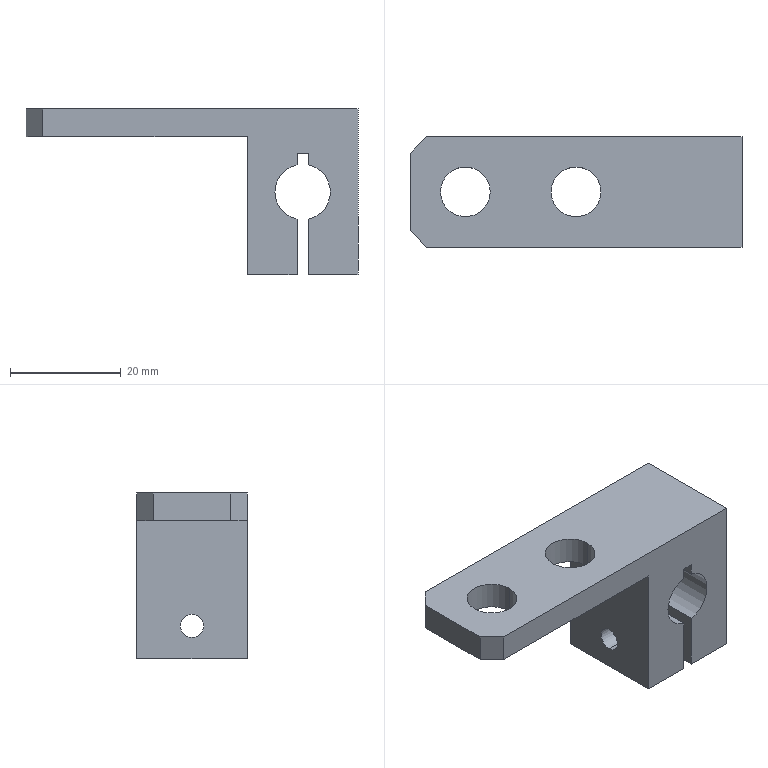Part | SolidWorks | features BaseBody 1 | 1 solid | 30 faces | box 60 x 20 x 30 mm | volume 12631 mm3 | plane 17 | cylinder 13 | commonest cylinder face diameters 10 x5 9 x4 4.2 x2 5.5 x2
STEP:
#1=CARTESIAN_POINT('',(24.6,0.,11.));
#2=VERTEX_POINT('',#1);
#3=CARTESIAN_POINT('',(24.6,0.,1.));
#4=VERTEX_POINT('',#3);
#5=CARTESIAN_POINT('',(24.6,0.,6.));
#6=DIRECTION('',(1.,0.,0.));
#7=DIRECTION('',(0.,0.,-1.));
#8=AXIS2_PLACEMENT_3D('',#5,#6,#7);
#9=CIRCLE('',#8,5.);
#10=EDGE_CURVE('',#2,#4,#9,.T.);
#11=ORIENTED_EDGE('',*,*,#10,.F.);
#12=CARTESIAN_POINT('',(30.,0.,11.));
#13=VERTEX_POINT('',#12);
#14=CARTESIAN_POINT('',(30.,0.,11.));
#15=DIRECTION('',(1.,0.,0.));
#16=VECTOR('',#15,1000.);
#17=LINE('',#14,#16);
#18=EDGE_CURVE('',#2,#13,#17,.T.);
#19=ORIENTED_EDGE('',*,*,#18,.T.);
#20=CARTESIAN_POINT('',(30.,0.,1.));
#21=VERTEX_POINT('',#20);
#22=CARTESIAN_POINT('',(30.,0.,6.));
#23=DIRECTION('',(1.,0.,0.));
#24=DIRECTION('',(0.,0.,-1.));
#25=AXIS2_PLACEMENT_3D('',#22,#23,#24);
#26=CIRCLE('',#25,5.);
#27=EDGE_CURVE('',#13,#21,#26,.T.);
#28=ORIENTED_EDGE('',*,*,#27,.T.);
#29=CARTESIAN_POINT('',(30.,0.,1.));
#30=DIRECTION('',(1.,0.,0.));
#31=VECTOR('',#30,1000.);
#32=LINE('',#29,#31);
#33=EDGE_CURVE('',#4,#21,#32,.T.);
#34=ORIENTED_EDGE('',*,*,#33,.F.);
#35=EDGE_LOOP('',(#11,#19,#28,#34));
#36=FACE_OUTER_BOUND('',#35,.T.);
#37=CARTESIAN_POINT('',(30.,0.,6.));
#38=DIRECTION('',(1.,0.,0.));
#39=DIRECTION('',(0.,0.,-1.));
#40=AXIS2_PLACEMENT_3D('',#37,#38,#39);
#41=CYLINDRICAL_SURFACE('',#40,5.);
#42=ADVANCED_FACE('',(#36),#41,.F.);
#43=CARTESIAN_POINT('',(21.,0.,3.25));
#44=VERTEX_POINT('',#43);
#45=CARTESIAN_POINT('',(21.,0.,8.75));
#46=VERTEX_POINT('',#45);
#47=CARTESIAN_POINT('',(21.,0.,6.));
#48=DIRECTION('',(-1.,0.,0.));
#49=DIRECTION('',(0.,1.,0.));
#50=AXIS2_PLACEMENT_3D('',#47,#48,#49);
#51=CIRCLE('',#50,2.75);
#52=EDGE_CURVE('',#44,#46,#51,.T.);
#53=ORIENTED_EDGE('',*,*,#52,.T.);
#54=CARTESIAN_POINT('',(24.6,0.,8.75));
#55=VERTEX_POINT('',#54);
#56=CARTESIAN_POINT('',(30.,0.,8.75));
#57=DIRECTION('',(1.,0.,0.));
#58=VECTOR('',#57,1000.);
#59=LINE('',#56,#58);
#60=EDGE_CURVE('',#46,#55,#59,.T.);
#61=ORIENTED_EDGE('',*,*,#60,.T.);
#62=CARTESIAN_POINT('',(24.6,0.,3.25));
#63=VERTEX_POINT('',#62);
#64=CARTESIAN_POINT('',(24.6,0.,6.));
#65=DIRECTION('',(1.,0.,0.));
#66=DIRECTION('',(0.,0.,-1.));
#67=AXIS2_PLACEMENT_3D('',#64,#65,#66);
#68=CIRCLE('',#67,2.75);
#69=EDGE_CURVE('',#55,#63,#68,.T.);
#70=ORIENTED_EDGE('',*,*,#69,.T.);
#71=CARTESIAN_POINT('',(30.,0.,3.25));
#72=DIRECTION('',(1.,0.,0.));
#73=VECTOR('',#72,1000.);
#74=LINE('',#71,#73);
#75=EDGE_CURVE('',#44,#63,#74,.T.);
#76=ORIENTED_EDGE('',*,*,#75,.F.);
#77=EDGE_LOOP('',(#53,#61,#70,#76));
#78=FACE_OUTER_BOUND('',#77,.T.);
#79=CARTESIAN_POINT('',(30.,0.,6.));
#80=DIRECTION('',(1.,0.,0.));
#81=DIRECTION('',(0.,0.,-1.));
#82=AXIS2_PLACEMENT_3D('',#79,#80,#81);
#83=CYLINDRICAL_SURFACE('',#82,2.75);
#84=ADVANCED_FACE('',(#78),#83,.F.);
#85=CARTESIAN_POINT('',(10.,0.,8.1));
#86=VERTEX_POINT('',#85);
#87=CARTESIAN_POINT('',(10.,0.,3.9));
#88=VERTEX_POINT('',#87);
#89=CARTESIAN_POINT('',(10.,0.,6.));
#90=DIRECTION('',(1.,0.,0.));
#91=DIRECTION('',(0.,1.,0.));
#92=AXIS2_PLACEMENT_3D('',#89,#90,#91);
#93=CIRCLE('',#92,2.1);
#94=EDGE_CURVE('',#86,#88,#93,.T.);
#95=ORIENTED_EDGE('',*,*,#94,.F.);
#96=CARTESIAN_POINT('',(19.,0.,8.1));
#97=VERTEX_POINT('',#96);
#98=CARTESIAN_POINT('',(19.,0.,8.1));
#99=DIRECTION('',(1.,0.,0.));
#100=VECTOR('',#99,1000.);
#101=LINE('',#98,#100);
#102=EDGE_CURVE('',#86,#97,#101,.T.);
#103=ORIENTED_EDGE('',*,*,#102,.T.);
#104=CARTESIAN_POINT('',(19.,0.,3.9));
#105=VERTEX_POINT('',#104);
#106=CARTESIAN_POINT('',(19.,0.,6.));
#107=DIRECTION('',(1.,0.,0.));
#108=DIRECTION('',(0.,0.,-1.));
#109=AXIS2_PLACEMENT_3D('',#106,#107,#108);
#110=CIRCLE('',#109,2.1);
#111=EDGE_CURVE('',#97,#105,#110,.T.);
#112=ORIENTED_EDGE('',*,*,#111,.T.);
#113=CARTESIAN_POINT('',(19.,0.,3.9));
#114=DIRECTION('',(1.,0.,0.));
#115=VECTOR('',#114,1000.);
#116=LINE('',#113,#115);
#117=EDGE_CURVE('',#88,#105,#116,.T.);
#118=ORIENTED_EDGE('',*,*,#117,.F.);
#119=EDGE_LOOP('',(#95,#103,#112,#118));
#120=FACE_OUTER_BOUND('',#119,.T.);
#121=CARTESIAN_POINT('',(19.,0.,6.));
#122=DIRECTION('',(1.,0.,0.));
#123=DIRECTION('',(0.,0.,-1.));
#124=AXIS2_PLACEMENT_3D('',#121,#122,#123);
#125=CYLINDRICAL_SURFACE('',#124,2.1);
#126=ADVANCED_FACE('',(#120),#125,.F.);
#127=CARTESIAN_POINT('',(-24.5,0.,30.));
#128=VERTEX_POINT('',#127);
#129=CARTESIAN_POINT('',(-15.5,0.,30.));
#130=VERTEX_POINT('',#129);
#131=CARTESIAN_POINT('',(-20.,0.,30.));
#132=DIRECTION('',(0.,0.,1.));
#133=DIRECTION('',(1.,0.,0.));
#134=AXIS2_PLACEMENT_3D('',#131,#132,#133);
#135=CIRCLE('',#134,4.5);
#136=EDGE_CURVE('',#128,#130,#135,.T.);
#137=ORIENTED_EDGE('',*,*,#136,.T.);
#138=CARTESIAN_POINT('',(-15.5,0.,25.));
#139=VERTEX_POINT('',#138);
#140=CARTESIAN_POINT('',(-15.5,0.,25.));
#141=DIRECTION('',(0.,0.,-1.));
#142=VECTOR('',#141,1000.);
#143=LINE('',#140,#142);
#144=EDGE_CURVE('',#130,#139,#143,.T.);
#145=ORIENTED_EDGE('',*,*,#144,.T.);
#146=CARTESIAN_POINT('',(-24.5,0.,25.));
#147=VERTEX_POINT('',#146);
#148=CARTESIAN_POINT('',(-20.,0.,25.));
#149=DIRECTION('',(0.,0.,-1.));
#150=DIRECTION('',(-1.,0.,0.));
#151=AXIS2_PLACEMENT_3D('',#148,#149,#150);
#152=CIRCLE('',#151,4.5);
#153=EDGE_CURVE('',#139,#147,#152,.T.);
#154=ORIENTED_EDGE('',*,*,#153,.T.);
#155=CARTESIAN_POINT('',(-24.5,0.,25.));
#156=DIRECTION('',(0.,0.,-1.));
#157=VECTOR('',#156,1000.);
#158=LINE('',#155,#157);
#159=EDGE_CURVE('',#128,#147,#158,.T.);
#160=ORIENTED_EDGE('',*,*,#159,.F.);
#161=EDGE_LOOP('',(#137,#145,#154,#160));
#162=FACE_OUTER_BOUND('',#161,.T.);
#163=CARTESIAN_POINT('',(-20.,0.,25.));
#164=DIRECTION('',(0.,0.,-1.));
#165=DIRECTION('',(-1.,0.,0.));
#166=AXIS2_PLACEMENT_3D('',#163,#164,#165);
#167=CYLINDRICAL_SURFACE('',#166,4.5);
#168=ADVANCED_FACE('',(#162),#167,.F.);
#169=CARTESIAN_POINT('',(-4.5,0.,30.));
#170=VERTEX_POINT('',#169);
#171=CARTESIAN_POINT('',(4.5,0.,30.));
#172=VERTEX_POINT('',#171);
#173=CARTESIAN_POINT('',(0.,0.,30.));
#174=DIRECTION('',(0.,0.,1.));
#175=DIRECTION('',(1.,0.,0.));
#176=AXIS2_PLACEMENT_3D('',#173,#174,#175);
#177=CIRCLE('',#176,4.5);
#178=EDGE_CURVE('',#170,#172,#177,.T.);
#179=ORIENTED_EDGE('',*,*,#178,.T.);
#180=CARTESIAN_POINT('',(4.5,0.,25.));
#181=VERTEX_POINT('',#180);
#182=CARTESIAN_POINT('',(4.5,0.,25.));
#183=DIRECTION('',(0.,0.,-1.));
#184=VECTOR('',#183,1000.);
#185=LINE('',#182,#184);
#186=EDGE_CURVE('',#172,#181,#185,.T.);
#187=ORIENTED_EDGE('',*,*,#186,.T.);
#188=CARTESIAN_POINT('',(-4.5,0.,25.));
#189=VERTEX_POINT('',#188);
#190=CARTESIAN_POINT('',(0.,0.,25.));
#191=DIRECTION('',(0.,0.,-1.));
#192=DIRECTION('',(-1.,0.,0.));
#193=AXIS2_PLACEMENT_3D('',#190,#191,#192);
#194=CIRCLE('',#193,4.5);
#195=EDGE_CURVE('',#181,#189,#194,.T.);
#196=ORIENTED_EDGE('',*,*,#195,.T.);
#197=CARTESIAN_POINT('',(-4.5,0.,25.));
#198=DIRECTION('',(0.,0.,-1.));
#199=VECTOR('',#198,1000.);
#200=LINE('',#197,#199);
#201=EDGE_CURVE('',#170,#189,#200,.T.);
#202=ORIENTED_EDGE('',*,*,#201,.F.);
#203=EDGE_LOOP('',(#179,#187,#196,#202));
#204=FACE_OUTER_BOUND('',#203,.T.);
#205=CARTESIAN_POINT('',(0.,0.,25.));
#206=DIRECTION('',(0.,0.,-1.));
#207=DIRECTION('',(-1.,0.,0.));
#208=AXIS2_PLACEMENT_3D('',#205,#206,#207);
#209=CYLINDRICAL_SURFACE('',#208,4.5);
#210=ADVANCED_FACE('',(#204),#209,.F.);
#211=CARTESIAN_POINT('',(15.,-10.,15.));
#212=VERTEX_POINT('',#211);
#213=CARTESIAN_POINT('',(19.,-10.,19.899));
#214=VERTEX_POINT('',#213);
#215=CARTESIAN_POINT('',(20.,-10.,15.));
#216=DIRECTION('',(0.,1.,0.));
#217=DIRECTION('',(-1.,0.,0.));
#218=AXIS2_PLACEMENT_3D('',#215,#216,#217);
#219=CIRCLE('',#218,5.);
#220=EDGE_CURVE('',#212,#214,#219,.T.);
#221=ORIENTED_EDGE('',*,*,#220,.F.);
#222=CARTESIAN_POINT('',(15.,10.,15.));
#223=VERTEX_POINT('',#222);
#224=CARTESIAN_POINT('',(15.,-10.,15.));
#225=DIRECTION('',(0.,1.,0.));
#226=VECTOR('',#225,1000.);
#227=LINE('',#224,#226);
#228=EDGE_CURVE('',#212,#223,#227,.T.);
#229=ORIENTED_EDGE('',*,*,#228,.T.);
#230=CARTESIAN_POINT('',(19.,10.,19.899));
#231=VERTEX_POINT('',#230);
#232=CARTESIAN_POINT('',(20.,10.,15.));
#233=DIRECTION('',(0.,1.,0.));
#234=DIRECTION('',(-1.,0.,0.));
#235=AXIS2_PLACEMENT_3D('',#232,#233,#234);
#236=CIRCLE('',#235,5.);
#237=EDGE_CURVE('',#223,#231,#236,.T.);
#238=ORIENTED_EDGE('',*,*,#237,.T.);
#239=CARTESIAN_POINT('',(19.,-10.,19.899));
#240=DIRECTION('',(0.,-1.,0.));
#241=VECTOR('',#240,1000.);
#242=LINE('',#239,#241);
#243=EDGE_CURVE('',#231,#214,#242,.T.);
#244=ORIENTED_EDGE('',*,*,#243,.T.);
#245=EDGE_LOOP('',(#221,#229,#238,#244));
#246=FACE_OUTER_BOUND('',#245,.T.);
#247=CARTESIAN_POINT('',(20.,-10.,15.));
#248=DIRECTION('',(0.,1.,0.));
#249=DIRECTION('',(-1.,0.,0.));
#250=AXIS2_PLACEMENT_3D('',#247,#248,#249);
#251=CYLINDRICAL_SURFACE('',#250,5.);
#252=ADVANCED_FACE('',(#246),#251,.F.);
#253=CARTESIAN_POINT('',(21.,10.,0.));
#254=VERTEX_POINT('',#253);
#255=CARTESIAN_POINT('',(21.,10.,10.101));
#256=VERTEX_POINT('',#255);
#257=CARTESIAN_POINT('',(21.,10.,22.));
#258=DIRECTION('',(0.,0.,1.));
#259=VECTOR('',#258,1000.);
#260=LINE('',#257,#259);
#261=EDGE_CURVE('',#254,#256,#260,.T.);
#262=ORIENTED_EDGE('',*,*,#261,.F.);
#263=CARTESIAN_POINT('',(21.,-10.,0.));
#264=VERTEX_POINT('',#263);
#265=CARTESIAN_POINT('',(21.,10.,0.));
#266=DIRECTION('',(0.,-1.,0.));
#267=VECTOR('',#266,1000.);
#268=LINE('',#265,#267);
#269=EDGE_CURVE('',#254,#264,#268,.T.);
#270=ORIENTED_EDGE('',*,*,#269,.T.);
#271=CARTESIAN_POINT('',(21.,-10.,10.101));
#272=VERTEX_POINT('',#271);
#273=CARTESIAN_POINT('',(21.,-10.,22.));
#274=DIRECTION('',(0.,0.,1.));
#275=VECTOR('',#274,1000.);
#276=LINE('',#273,#275);
#277=EDGE_CURVE('',#264,#272,#276,.T.);
#278=ORIENTED_EDGE('',*,*,#277,.T.);
#279=CARTESIAN_POINT('',(21.,-10.,10.101));
#280=DIRECTION('',(0.,-1.,0.));
#281=VECTOR('',#280,1000.);
#282=LINE('',#279,#281);
#283=EDGE_CURVE('',#256,#272,#282,.T.);
#284=ORIENTED_EDGE('',*,*,#283,.F.);
#285=EDGE_LOOP('',(#262,#270,#278,#284));
#286=FACE_OUTER_BOUND('',#285,.T.);
#287=ORIENTED_EDGE('',*,*,#52,.F.);
#288=CARTESIAN_POINT('',(21.,0.,6.));
#289=DIRECTION('',(-1.,0.,0.));
#290=DIRECTION('',(0.,1.,0.));
#291=AXIS2_PLACEMENT_3D('',#288,#289,#290);
#292=CIRCLE('',#291,2.75);
#293=EDGE_CURVE('',#46,#44,#292,.T.);
#294=ORIENTED_EDGE('',*,*,#293,.F.);
#295=EDGE_LOOP('',(#287,#294));
#296=FACE_BOUND('',#295,.T.);
#297=CARTESIAN_POINT('',(21.,10.,22.));
#298=DIRECTION('',(1.,0.,0.));
#299=DIRECTION('',(0.,1.,0.));
#300=AXIS2_PLACEMENT_3D('',#297,#298,#299);
#301=PLANE('',#300);
#302=ADVANCED_FACE('',(#286,#296),#301,.F.);
#303=CARTESIAN_POINT('',(19.,10.,0.));
#304=VERTEX_POINT('',#303);
#305=CARTESIAN_POINT('',(10.,10.,0.));
#306=VERTEX_POINT('',#305);
#307=CARTESIAN_POINT('',(30.,10.,0.));
#308=DIRECTION('',(-1.,0.,0.));
#309=VECTOR('',#308,1000.);
#310=LINE('',#307,#309);
#311=EDGE_CURVE('',#304,#306,#310,.T.);
#312=ORIENTED_EDGE('',*,*,#311,.F.);
#313=CARTESIAN_POINT('',(19.,-10.,0.));
#314=VERTEX_POINT('',#313);
#315=CARTESIAN_POINT('',(19.,10.,0.));
#316=DIRECTION('',(0.,-1.,0.));
#317=VECTOR('',#316,1000.);
#318=LINE('',#315,#317);
#319=EDGE_CURVE('',#304,#314,#318,.T.);
#320=ORIENTED_EDGE('',*,*,#319,.T.);
#321=CARTESIAN_POINT('',(10.,-10.,0.));
#322=VERTEX_POINT('',#321);
#323=CARTESIAN_POINT('',(30.,-10.,0.));
#324=DIRECTION('',(1.,0.,0.));
#325=VECTOR('',#324,1000.);
#326=LINE('',#323,#325);
#327=EDGE_CURVE('',#322,#314,#326,.T.);
#328=ORIENTED_EDGE('',*,*,#327,.F.);
#329=CARTESIAN_POINT('',(10.,-10.,0.));
#330=DIRECTION('',(0.,1.,0.));
#331=VECTOR('',#330,1000.);
#332=LINE('',#329,#331);
#333=EDGE_CURVE('',#322,#306,#332,.T.);
#334=ORIENTED_EDGE('',*,*,#333,.T.);
#335=EDGE_LOOP('',(#312,#320,#328,#334));
#336=FACE_OUTER_BOUND('',#335,.T.);
#337=CARTESIAN_POINT('',(0.,0.,0.));
#338=DIRECTION('',(0.,0.,1.));
#339=DIRECTION('',(1.,0.,0.));
#340=AXIS2_PLACEMENT_3D('',#337,#338,#339);
#341=PLANE('',#340);
#342=ADVANCED_FACE('',(#336),#341,.F.);
#343=ORIENTED_EDGE('',*,*,#228,.F.);
#344=CARTESIAN_POINT('',(19.,-10.,10.101));
#345=VERTEX_POINT('',#344);
#346=CARTESIAN_POINT('',(20.,-10.,15.));
#347=DIRECTION('',(0.,1.,0.));
#348=DIRECTION('',(-1.,0.,0.));
#349=AXIS2_PLACEMENT_3D('',#346,#347,#348);
#350=CIRCLE('',#349,5.);
#351=EDGE_CURVE('',#345,#212,#350,.T.);
#352=ORIENTED_EDGE('',*,*,#351,.F.);
#353=CARTESIAN_POINT('',(19.,10.,10.101));
#354=VERTEX_POINT('',#353);
#355=CARTESIAN_POINT('',(19.,-10.,10.101));
#356=DIRECTION('',(0.,1.,0.));
#357=VECTOR('',#356,1000.);
#358=LINE('',#355,#357);
#359=EDGE_CURVE('',#345,#354,#358,.T.);
#360=ORIENTED_EDGE('',*,*,#359,.T.);
#361=CARTESIAN_POINT('',(20.,10.,15.));
#362=DIRECTION('',(0.,1.,0.));
#363=DIRECTION('',(-1.,0.,0.));
#364=AXIS2_PLACEMENT_3D('',#361,#362,#363);
#365=CIRCLE('',#364,5.);
#366=EDGE_CURVE('',#354,#223,#365,.T.);
#367=ORIENTED_EDGE('',*,*,#366,.T.);
#368=EDGE_LOOP('',(#343,#352,#360,#367));
#369=FACE_OUTER_BOUND('',#368,.T.);
#370=CARTESIAN_POINT('',(20.,-10.,15.));
#371=DIRECTION('',(0.,1.,0.));
#372=DIRECTION('',(-1.,0.,0.));
#373=AXIS2_PLACEMENT_3D('',#370,#371,#372);
#374=CYLINDRICAL_SURFACE('',#373,5.);
#375=ADVANCED_FACE('',(#369),#374,.F.);
#376=CARTESIAN_POINT('',(-30.,-7.,25.));
#377=VERTEX_POINT('',#376);
#378=CARTESIAN_POINT('',(-30.,7.,25.));
#379=VERTEX_POINT('',#378);
#380=CARTESIAN_POINT('',(-30.,-10.,25.));
#381=DIRECTION('',(0.,1.,0.));
#382=VECTOR('',#381,1000.);
#383=LINE('',#380,#382);
#384=EDGE_CURVE('',#377,#379,#383,.T.);
#385=ORIENTED_EDGE('',*,*,#384,.F.);
#386=CARTESIAN_POINT('',(-30.,-7.,30.));
#387=VERTEX_POINT('',#386);
#388=CARTESIAN_POINT('',(-30.,-7.,30.));
#389=DIRECTION('',(0.,0.,1.));
#390=VECTOR('',#389,1000.);
#391=LINE('',#388,#390);
#392=EDGE_CURVE('',#377,#387,#391,.T.);
#393=ORIENTED_EDGE('',*,*,#392,.T.);
#394=CARTESIAN_POINT('',(-30.,7.,30.));
#395=VERTEX_POINT('',#394);
#396=CARTESIAN_POINT('',(-30.,-10.,30.));
#397=DIRECTION('',(0.,-1.,0.));
#398=VECTOR('',#397,1000.);
#399=LINE('',#396,#398);
#400=EDGE_CURVE('',#395,#387,#399,.T.);
#401=ORIENTED_EDGE('',*,*,#400,.F.);
#402=CARTESIAN_POINT('',(-30.,7.,30.));
#403=DIRECTION('',(0.,0.,-1.));
#404=VECTOR('',#403,1000.);
#405=LINE('',#402,#404);
#406=EDGE_CURVE('',#395,#379,#405,.T.);
#407=ORIENTED_EDGE('',*,*,#406,.T.);
#408=EDGE_LOOP('',(#385,#393,#401,#407));
#409=FACE_OUTER_BOUND('',#408,.T.);
#410=CARTESIAN_POINT('',(-30.,-10.,30.));
#411=DIRECTION('',(1.,0.,0.));
#412=DIRECTION('',(0.,0.,-1.));
#413=AXIS2_PLACEMENT_3D('',#410,#411,#412);
#414=PLANE('',#413);
#415=ADVANCED_FACE('',(#409),#414,.F.);
#416=ORIENTED_EDGE('',*,*,#327,.T.);
#417=CARTESIAN_POINT('',(19.,-10.,22.));
#418=DIRECTION('',(0.,0.,-1.));
#419=VECTOR('',#418,1000.);
#420=LINE('',#417,#419);
#421=EDGE_CURVE('',#345,#314,#420,.T.);
#422=ORIENTED_EDGE('',*,*,#421,.F.);
#423=ORIENTED_EDGE('',*,*,#351,.T.);
#424=ORIENTED_EDGE('',*,*,#220,.T.);
#425=CARTESIAN_POINT('',(19.,-10.,22.));
#426=VERTEX_POINT('',#425);
#427=CARTESIAN_POINT('',(19.,-10.,22.));
#428=DIRECTION('',(0.,0.,-1.));
#429=VECTOR('',#428,1000.);
#430=LINE('',#427,#429);
#431=EDGE_CURVE('',#426,#214,#430,.T.);
#432=ORIENTED_EDGE('',*,*,#431,.F.);
#433=CARTESIAN_POINT('',(21.,-10.,22.));
#434=VERTEX_POINT('',#433);
#435=CARTESIAN_POINT('',(19.,-10.,22.));
#436=DIRECTION('',(-1.,0.,0.));
#437=VECTOR('',#436,1000.);
#438=LINE('',#435,#437);
#439=EDGE_CURVE('',#434,#426,#438,.T.);
#440=ORIENTED_EDGE('',*,*,#439,.F.);
#441=CARTESIAN_POINT('',(21.,-10.,19.899));
#442=VERTEX_POINT('',#441);
#443=CARTESIAN_POINT('',(21.,-10.,22.));
#444=DIRECTION('',(0.,0.,1.));
#445=VECTOR('',#444,1000.);
#446=LINE('',#443,#445);
#447=EDGE_CURVE('',#442,#434,#446,.T.);
#448=ORIENTED_EDGE('',*,*,#447,.F.);
#449=CARTESIAN_POINT('',(20.,-10.,15.));
#450=DIRECTION('',(0.,1.,0.));
#451=DIRECTION('',(-1.,0.,0.));
#452=AXIS2_PLACEMENT_3D('',#449,#450,#451);
#453=CIRCLE('',#452,5.);
#454=EDGE_CURVE('',#442,#272,#453,.T.);
#455=ORIENTED_EDGE('',*,*,#454,.T.);
#456=ORIENTED_EDGE('',*,*,#277,.F.);
#457=CARTESIAN_POINT('',(30.,-10.,0.));
#458=VERTEX_POINT('',#457);
#459=CARTESIAN_POINT('',(30.,-10.,0.));
#460=DIRECTION('',(1.,0.,0.));
#461=VECTOR('',#460,1000.);
#462=LINE('',#459,#461);
#463=EDGE_CURVE('',#264,#458,#462,.T.);
#464=ORIENTED_EDGE('',*,*,#463,.T.);
#465=CARTESIAN_POINT('',(30.,-10.,30.));
#466=VERTEX_POINT('',#465);
#467=CARTESIAN_POINT('',(30.,-10.,30.));
#468=DIRECTION('',(0.,0.,-1.));
#469=VECTOR('',#468,1000.);
#470=LINE('',#467,#469);
#471=EDGE_CURVE('',#466,#458,#470,.T.);
#472=ORIENTED_EDGE('',*,*,#471,.F.);
#473=CARTESIAN_POINT('',(-27.,-10.,30.));
#474=VERTEX_POINT('',#473);
#475=CARTESIAN_POINT('',(30.,-10.,30.));
#476=DIRECTION('',(1.,0.,0.));
#477=VECTOR('',#476,1000.);
#478=LINE('',#475,#477);
#479=EDGE_CURVE('',#474,#466,#478,.T.);
#480=ORIENTED_EDGE('',*,*,#479,.F.);
#481=CARTESIAN_POINT('',(-27.,-10.,25.));
#482=VERTEX_POINT('',#481);
#483=CARTESIAN_POINT('',(-27.,-10.,30.));
#484=DIRECTION('',(0.,0.,-1.));
#485=VECTOR('',#484,1000.);
#486=LINE('',#483,#485);
#487=EDGE_CURVE('',#474,#482,#486,.T.);
#488=ORIENTED_EDGE('',*,*,#487,.T.);
#489=CARTESIAN_POINT('',(10.,-10.,25.));
#490=VERTEX_POINT('',#489);
#491=CARTESIAN_POINT('',(-30.,-10.,25.));
#492=DIRECTION('',(1.,0.,0.));
#493=VECTOR('',#492,1000.);
#494=LINE('',#491,#493);
#495=EDGE_CURVE('',#482,#490,#494,.T.);
#496=ORIENTED_EDGE('',*,*,#495,.T.);
#497=CARTESIAN_POINT('',(10.,-10.,25.));
#498=DIRECTION('',(0.,0.,-1.));
#499=VECTOR('',#498,1000.);
#500=LINE('',#497,#499);
#501=EDGE_CURVE('',#490,#322,#500,.T.);
#502=ORIENTED_EDGE('',*,*,#501,.T.);
#503=EDGE_LOOP('',(#416,#422,#423,#424,#432,#440,#448,#455,#456,#464,#472,#480,#488,#496,#502));
#504=FACE_OUTER_BOUND('',#503,.T.);
#505=CARTESIAN_POINT('',(30.,-10.,30.));
#506=DIRECTION('',(0.,1.,0.));
#507=DIRECTION('',(-1.,0.,0.));
#508=AXIS2_PLACEMENT_3D('',#505,#506,#507);
#509=PLANE('',#508);
#510=ADVANCED_FACE('',(#504),#509,.F.);
#511=CARTESIAN_POINT('',(30.,0.,6.));
#512=DIRECTION('',(1.,0.,0.));
#513=DIRECTION('',(0.,0.,-1.));
#514=AXIS2_PLACEMENT_3D('',#511,#512,#513);
#515=CIRCLE('',#514,5.);
#516=EDGE_CURVE('',#21,#13,#515,.T.);
#517=ORIENTED_EDGE('',*,*,#516,.F.);
#518=ORIENTED_EDGE('',*,*,#27,.F.);
#519=EDGE_LOOP('',(#517,#518));
#520=FACE_BOUND('',#519,.T.);
#521=CARTESIAN_POINT('',(30.,10.,0.));
#522=VERTEX_POINT('',#521);
#523=CARTESIAN_POINT('',(30.,-10.,0.));
#524=DIRECTION('',(0.,1.,0.));
#525=VECTOR('',#524,1000.);
#526=LINE('',#523,#525);
#527=EDGE_CURVE('',#458,#522,#526,.T.);
#528=ORIENTED_EDGE('',*,*,#527,.T.);
#529=CARTESIAN_POINT('',(30.,10.,30.));
#530=VERTEX_POINT('',#529);
#531=CARTESIAN_POINT('',(30.,10.,30.));
#532=DIRECTION('',(0.,0.,-1.));
#533=VECTOR('',#532,1000.);
#534=LINE('',#531,#533);
#535=EDGE_CURVE('',#530,#522,#534,.T.);
#536=ORIENTED_EDGE('',*,*,#535,.F.);
#537=CARTESIAN_POINT('',(30.,-10.,30.));
#538=DIRECTION('',(0.,1.,0.));
#539=VECTOR('',#538,1000.);
#540=LINE('',#537,#539);
#541=EDGE_CURVE('',#466,#530,#540,.T.);
#542=ORIENTED_EDGE('',*,*,#541,.F.);
#543=ORIENTED_EDGE('',*,*,#471,.T.);
#544=EDGE_LOOP('',(#528,#536,#542,#543));
#545=FACE_OUTER_BOUND('',#544,.T.);
#546=CARTESIAN_POINT('',(30.,-10.,30.));
#547=DIRECTION('',(-1.,0.,0.));
#548=DIRECTION('',(0.,0.,1.));
#549=AXIS2_PLACEMENT_3D('',#546,#547,#548);
#550=PLANE('',#549);
#551=ADVANCED_FACE('',(#520,#545),#550,.F.);
#552=ORIENTED_EDGE('',*,*,#366,.F.);
#553=CARTESIAN_POINT('',(19.,10.,22.));
#554=DIRECTION('',(0.,0.,-1.));
#555=VECTOR('',#554,1000.);
#556=LINE('',#553,#555);
#557=EDGE_CURVE('',#354,#304,#556,.T.);
#558=ORIENTED_EDGE('',*,*,#557,.T.);
#559=ORIENTED_EDGE('',*,*,#311,.T.);
#560=CARTESIAN_POINT('',(10.,10.,25.));
#561=VERTEX_POINT('',#560);
#562=CARTESIAN_POINT('',(10.,10.,25.));
#563=DIRECTION('',(0.,0.,-1.));
#564=VECTOR('',#563,1000.);
#565=LINE('',#562,#564);
#566=EDGE_CURVE('',#561,#306,#565,.T.);
#567=ORIENTED_EDGE('',*,*,#566,.F.);
#568=CARTESIAN_POINT('',(-27.,10.,25.));
#569=VERTEX_POINT('',#568);
#570=CARTESIAN_POINT('',(-30.,10.,25.));
#571=DIRECTION('',(1.,0.,0.));
#572=VECTOR('',#571,1000.);
#573=LINE('',#570,#572);
#574=EDGE_CURVE('',#569,#561,#573,.T.);
#575=ORIENTED_EDGE('',*,*,#574,.F.);
#576=CARTESIAN_POINT('',(-27.,10.,30.));
#577=VERTEX_POINT('',#576);
#578=CARTESIAN_POINT('',(-27.,10.,30.));
#579=DIRECTION('',(0.,0.,1.));
#580=VECTOR('',#579,1000.);
#581=LINE('',#578,#580);
#582=EDGE_CURVE('',#569,#577,#581,.T.);
#583=ORIENTED_EDGE('',*,*,#582,.T.);
#584=CARTESIAN_POINT('',(30.,10.,30.));
#585=DIRECTION('',(-1.,0.,0.));
#586=VECTOR('',#585,1000.);
#587=LINE('',#584,#586);
#588=EDGE_CURVE('',#530,#577,#587,.T.);
#589=ORIENTED_EDGE('',*,*,#588,.F.);
#590=ORIENTED_EDGE('',*,*,#535,.T.);
#591=CARTESIAN_POINT('',(30.,10.,0.));
#592=DIRECTION('',(-1.,0.,0.));
#593=VECTOR('',#592,1000.);
#594=LINE('',#591,#593);
#595=EDGE_CURVE('',#522,#254,#594,.T.);
#596=ORIENTED_EDGE('',*,*,#595,.T.);
#597=ORIENTED_EDGE('',*,*,#261,.T.);
#598=CARTESIAN_POINT('',(21.,10.,19.899));
#599=VERTEX_POINT('',#598);
#600=CARTESIAN_POINT('',(20.,10.,15.));
#601=DIRECTION('',(0.,1.,0.));
#602=DIRECTION('',(-1.,0.,0.));
#603=AXIS2_PLACEMENT_3D('',#600,#601,#602);
#604=CIRCLE('',#603,5.);
#605=EDGE_CURVE('',#599,#256,#604,.T.);
#606=ORIENTED_EDGE('',*,*,#605,.F.);
#607=CARTESIAN_POINT('',(21.,10.,22.));
#608=VERTEX_POINT('',#607);
#609=CARTESIAN_POINT('',(21.,10.,22.));
#610=DIRECTION('',(0.,0.,1.));
#611=VECTOR('',#610,1000.);
#612=LINE('',#609,#611);
#613=EDGE_CURVE('',#599,#608,#612,.T.);
#614=ORIENTED_EDGE('',*,*,#613,.T.);
#615=CARTESIAN_POINT('',(19.,10.,22.));
#616=VERTEX_POINT('',#615);
#617=CARTESIAN_POINT('',(19.,10.,22.));
#618=DIRECTION('',(-1.,0.,0.));
#619=VECTOR('',#618,1000.);
#620=LINE('',#617,#619);
#621=EDGE_CURVE('',#608,#616,#620,.T.);
#622=ORIENTED_EDGE('',*,*,#621,.T.);
#623=CARTESIAN_POINT('',(19.,10.,22.));
#624=DIRECTION('',(0.,0.,-1.));
#625=VECTOR('',#624,1000.);
#626=LINE('',#623,#625);
#627=EDGE_CURVE('',#616,#231,#626,.T.);
#628=ORIENTED_EDGE('',*,*,#627,.T.);
#629=ORIENTED_EDGE('',*,*,#237,.F.);
#630=EDGE_LOOP('',(#552,#558,#559,#567,#575,#583,#589,#590,#596,#597,#606,#614,#622,#628,#629));
#631=FACE_OUTER_BOUND('',#630,.T.);
#632=CARTESIAN_POINT('',(30.,10.,30.));
#633=DIRECTION('',(0.,-1.,0.));
#634=DIRECTION('',(1.,0.,0.));
#635=AXIS2_PLACEMENT_3D('',#632,#633,#634);
#636=PLANE('',#635);
#637=ADVANCED_FACE('',(#631),#636,.F.);
#638=ORIENTED_EDGE('',*,*,#136,.F.);
#639=CARTESIAN_POINT('',(-20.,0.,30.));
#640=DIRECTION('',(0.,0.,1.));
#641=DIRECTION('',(1.,0.,0.));
#642=AXIS2_PLACEMENT_3D('',#639,#640,#641);
#643=CIRCLE('',#642,4.5);
#644=EDGE_CURVE('',#130,#128,#643,.T.);
#645=ORIENTED_EDGE('',*,*,#644,.F.);
#646=EDGE_LOOP('',(#638,#645));
#647=FACE_BOUND('',#646,.T.);
#648=ORIENTED_EDGE('',*,*,#178,.F.);
#649=CARTESIAN_POINT('',(0.,0.,30.));
#650=DIRECTION('',(0.,0.,1.));
#651=DIRECTION('',(1.,0.,0.));
#652=AXIS2_PLACEMENT_3D('',#649,#650,#651);
#653=CIRCLE('',#652,4.5);
#654=EDGE_CURVE('',#172,#170,#653,.T.);
#655=ORIENTED_EDGE('',*,*,#654,.F.);
#656=EDGE_LOOP('',(#648,#655));
#657=FACE_BOUND('',#656,.T.);
#658=ORIENTED_EDGE('',*,*,#400,.T.);
#659=CARTESIAN_POINT('',(-18.5,-18.5,30.));
#660=DIRECTION('',(0.7071,-0.7071,0.));
#661=VECTOR('',#660,1000.);
#662=LINE('',#659,#661);
#663=EDGE_CURVE('',#387,#474,#662,.T.);
#664=ORIENTED_EDGE('',*,*,#663,.T.);
#665=ORIENTED_EDGE('',*,*,#479,.T.);
#666=ORIENTED_EDGE('',*,*,#541,.T.);
#667=ORIENTED_EDGE('',*,*,#588,.T.);
#668=CARTESIAN_POINT('',(-18.5,18.5,30.));
#669=DIRECTION('',(-0.7071,-0.7071,0.));
#670=VECTOR('',#669,1000.);
#671=LINE('',#668,#670);
#672=EDGE_CURVE('',#577,#395,#671,.T.);
#673=ORIENTED_EDGE('',*,*,#672,.T.);
#674=EDGE_LOOP('',(#658,#664,#665,#666,#667,#673));
#675=FACE_OUTER_BOUND('',#674,.T.);
#676=CARTESIAN_POINT('',(0.,0.,30.));
#677=DIRECTION('',(0.,0.,1.));
#678=DIRECTION('',(1.,0.,0.));
#679=AXIS2_PLACEMENT_3D('',#676,#677,#678);
#680=PLANE('',#679);
#681=ADVANCED_FACE('',(#647,#657,#675),#680,.T.);
#682=ORIENTED_EDGE('',*,*,#463,.F.);
#683=ORIENTED_EDGE('',*,*,#269,.F.);
#684=ORIENTED_EDGE('',*,*,#595,.F.);
#685=ORIENTED_EDGE('',*,*,#527,.F.);
#686=EDGE_LOOP('',(#682,#683,#684,#685));
#687=FACE_OUTER_BOUND('',#686,.T.);
#688=CARTESIAN_POINT('',(0.,0.,0.));
#689=DIRECTION('',(0.,0.,1.));
#690=DIRECTION('',(1.,0.,0.));
#691=AXIS2_PLACEMENT_3D('',#688,#689,#690);
#692=PLANE('',#691);
#693=ADVANCED_FACE('',(#687),#692,.F.);
#694=CARTESIAN_POINT('',(10.,0.,6.));
#695=DIRECTION('',(1.,0.,0.));
#696=DIRECTION('',(0.,1.,0.));
#697=AXIS2_PLACEMENT_3D('',#694,#695,#696);
#698=CIRCLE('',#697,2.1);
#699=EDGE_CURVE('',#88,#86,#698,.T.);
#700=ORIENTED_EDGE('',*,*,#699,.T.);
#701=ORIENTED_EDGE('',*,*,#94,.T.);
#702=EDGE_LOOP('',(#700,#701));
#703=FACE_BOUND('',#702,.T.);
#704=ORIENTED_EDGE('',*,*,#566,.T.);
#705=ORIENTED_EDGE('',*,*,#333,.F.);
#706=ORIENTED_EDGE('',*,*,#501,.F.);
#707=CARTESIAN_POINT('',(10.,-10.,25.));
#708=DIRECTION('',(0.,1.,0.));
#709=VECTOR('',#708,1000.);
#710=LINE('',#707,#709);
#711=EDGE_CURVE('',#490,#561,#710,.T.);
#712=ORIENTED_EDGE('',*,*,#711,.T.);
#713=EDGE_LOOP('',(#704,#705,#706,#712));
#714=FACE_OUTER_BOUND('',#713,.T.);
#715=CARTESIAN_POINT('',(10.,-10.,25.));
#716=DIRECTION('',(1.,0.,0.));
#717=DIRECTION('',(0.,1.,0.));
#718=AXIS2_PLACEMENT_3D('',#715,#716,#717);
#719=PLANE('',#718);
#720=ADVANCED_FACE('',(#703,#714),#719,.F.);
#721=CARTESIAN_POINT('',(-20.,0.,25.));
#722=DIRECTION('',(0.,0.,-1.));
#723=DIRECTION('',(-1.,0.,0.));
#724=AXIS2_PLACEMENT_3D('',#721,#722,#723);
#725=CIRCLE('',#724,4.5);
#726=EDGE_CURVE('',#147,#139,#725,.T.);
#727=ORIENTED_EDGE('',*,*,#726,.F.);
#728=ORIENTED_EDGE('',*,*,#153,.F.);
#729=EDGE_LOOP('',(#727,#728));
#730=FACE_BOUND('',#729,.T.);
#731=CARTESIAN_POINT('',(0.,0.,25.));
#732=DIRECTION('',(0.,0.,-1.));
#733=DIRECTION('',(-1.,0.,0.));
#734=AXIS2_PLACEMENT_3D('',#731,#732,#733);
#735=CIRCLE('',#734,4.5);
#736=EDGE_CURVE('',#189,#181,#735,.T.);
#737=ORIENTED_EDGE('',*,*,#736,.F.);
#738=ORIENTED_EDGE('',*,*,#195,.F.);
#739=EDGE_LOOP('',(#737,#738));
#740=FACE_BOUND('',#739,.T.);
#741=ORIENTED_EDGE('',*,*,#495,.F.);
#742=CARTESIAN_POINT('',(-27.,-10.,25.));
#743=DIRECTION('',(-0.7071,0.7071,0.));
#744=VECTOR('',#743,1000.);
#745=LINE('',#742,#744);
#746=EDGE_CURVE('',#482,#377,#745,.T.);
#747=ORIENTED_EDGE('',*,*,#746,.T.);
#748=ORIENTED_EDGE('',*,*,#384,.T.);
#749=CARTESIAN_POINT('',(-30.,7.,25.));
#750=DIRECTION('',(0.7071,0.7071,0.));
#751=VECTOR('',#750,1000.);
#752=LINE('',#749,#751);
#753=EDGE_CURVE('',#379,#569,#752,.T.);
#754=ORIENTED_EDGE('',*,*,#753,.T.);
#755=ORIENTED_EDGE('',*,*,#574,.T.);
#756=ORIENTED_EDGE('',*,*,#711,.F.);
#757=EDGE_LOOP('',(#741,#747,#748,#754,#755,#756));
#758=FACE_OUTER_BOUND('',#757,.T.);
#759=CARTESIAN_POINT('',(-30.,-10.,25.));
#760=DIRECTION('',(0.,0.,1.));
#761=DIRECTION('',(1.,0.,0.));
#762=AXIS2_PLACEMENT_3D('',#759,#760,#761);
#763=PLANE('',#762);
#764=ADVANCED_FACE('',(#730,#740,#758),#763,.F.);
#765=ORIENTED_EDGE('',*,*,#605,.T.);
#766=ORIENTED_EDGE('',*,*,#283,.T.);
#767=ORIENTED_EDGE('',*,*,#454,.F.);
#768=CARTESIAN_POINT('',(21.,-10.,19.899));
#769=DIRECTION('',(0.,1.,0.));
#770=VECTOR('',#769,1000.);
#771=LINE('',#768,#770);
#772=EDGE_CURVE('',#442,#599,#771,.T.);
#773=ORIENTED_EDGE('',*,*,#772,.T.);
#774=EDGE_LOOP('',(#765,#766,#767,#773));
#775=FACE_OUTER_BOUND('',#774,.T.);
#776=CARTESIAN_POINT('',(20.,-10.,15.));
#777=DIRECTION('',(0.,1.,0.));
#778=DIRECTION('',(-1.,0.,0.));
#779=AXIS2_PLACEMENT_3D('',#776,#777,#778);
#780=CYLINDRICAL_SURFACE('',#779,5.);
#781=ADVANCED_FACE('',(#775),#780,.F.);
#782=ORIENTED_EDGE('',*,*,#663,.F.);
#783=ORIENTED_EDGE('',*,*,#392,.F.);
#784=ORIENTED_EDGE('',*,*,#746,.F.);
#785=ORIENTED_EDGE('',*,*,#487,.F.);
#786=EDGE_LOOP('',(#782,#783,#784,#785));
#787=FACE_OUTER_BOUND('',#786,.T.);
#788=CARTESIAN_POINT('',(-27.,-10.,30.));
#789=DIRECTION('',(0.7071,0.7071,0.));
#790=DIRECTION('',(0.,0.,-1.));
#791=AXIS2_PLACEMENT_3D('',#788,#789,#790);
#792=PLANE('',#791);
#793=ADVANCED_FACE('',(#787),#792,.F.);
#794=ORIENTED_EDGE('',*,*,#672,.F.);
#795=ORIENTED_EDGE('',*,*,#582,.F.);
#796=ORIENTED_EDGE('',*,*,#753,.F.);
#797=ORIENTED_EDGE('',*,*,#406,.F.);
#798=EDGE_LOOP('',(#794,#795,#796,#797));
#799=FACE_OUTER_BOUND('',#798,.T.);
#800=CARTESIAN_POINT('',(-30.,7.,30.));
#801=DIRECTION('',(0.7071,-0.7071,0.));
#802=DIRECTION('',(0.,0.,-1.));
#803=AXIS2_PLACEMENT_3D('',#800,#801,#802);
#804=PLANE('',#803);
#805=ADVANCED_FACE('',(#799),#804,.F.);
#806=ORIENTED_EDGE('',*,*,#186,.F.);
#807=ORIENTED_EDGE('',*,*,#654,.T.);
#808=ORIENTED_EDGE('',*,*,#201,.T.);
#809=ORIENTED_EDGE('',*,*,#736,.T.);
#810=EDGE_LOOP('',(#806,#807,#808,#809));
#811=FACE_OUTER_BOUND('',#810,.T.);
#812=CARTESIAN_POINT('',(0.,0.,25.));
#813=DIRECTION('',(0.,0.,-1.));
#814=DIRECTION('',(-1.,0.,0.));
#815=AXIS2_PLACEMENT_3D('',#812,#813,#814);
#816=CYLINDRICAL_SURFACE('',#815,4.5);
#817=ADVANCED_FACE('',(#811),#816,.F.);
#818=ORIENTED_EDGE('',*,*,#144,.F.);
#819=ORIENTED_EDGE('',*,*,#644,.T.);
#820=ORIENTED_EDGE('',*,*,#159,.T.);
#821=ORIENTED_EDGE('',*,*,#726,.T.);
#822=EDGE_LOOP('',(#818,#819,#820,#821));
#823=FACE_OUTER_BOUND('',#822,.T.);
#824=CARTESIAN_POINT('',(-20.,0.,25.));
#825=DIRECTION('',(0.,0.,-1.));
#826=DIRECTION('',(-1.,0.,0.));
#827=AXIS2_PLACEMENT_3D('',#824,#825,#826);
#828=CYLINDRICAL_SURFACE('',#827,4.5);
#829=ADVANCED_FACE('',(#823),#828,.F.);
#830=ORIENTED_EDGE('',*,*,#627,.F.);
#831=CARTESIAN_POINT('',(19.,10.,22.));
#832=DIRECTION('',(0.,-1.,0.));
#833=VECTOR('',#832,1000.);
#834=LINE('',#831,#833);
#835=EDGE_CURVE('',#616,#426,#834,.T.);
#836=ORIENTED_EDGE('',*,*,#835,.T.);
#837=ORIENTED_EDGE('',*,*,#431,.T.);
#838=ORIENTED_EDGE('',*,*,#243,.F.);
#839=EDGE_LOOP('',(#830,#836,#837,#838));
#840=FACE_OUTER_BOUND('',#839,.T.);
#841=CARTESIAN_POINT('',(19.,10.,22.));
#842=DIRECTION('',(-1.,0.,0.));
#843=DIRECTION('',(0.,0.,1.));
#844=AXIS2_PLACEMENT_3D('',#841,#842,#843);
#845=PLANE('',#844);
#846=ADVANCED_FACE('',(#840),#845,.F.);
#847=ORIENTED_EDGE('',*,*,#447,.T.);
#848=CARTESIAN_POINT('',(21.,10.,22.));
#849=DIRECTION('',(0.,-1.,0.));
#850=VECTOR('',#849,1000.);
#851=LINE('',#848,#850);
#852=EDGE_CURVE('',#608,#434,#851,.T.);
#853=ORIENTED_EDGE('',*,*,#852,.F.);
#854=ORIENTED_EDGE('',*,*,#613,.F.);
#855=ORIENTED_EDGE('',*,*,#772,.F.);
#856=EDGE_LOOP('',(#847,#853,#854,#855));
#857=FACE_OUTER_BOUND('',#856,.T.);
#858=CARTESIAN_POINT('',(21.,10.,22.));
#859=DIRECTION('',(1.,0.,0.));
#860=DIRECTION('',(0.,1.,0.));
#861=AXIS2_PLACEMENT_3D('',#858,#859,#860);
#862=PLANE('',#861);
#863=ADVANCED_FACE('',(#857),#862,.F.);
#864=ORIENTED_EDGE('',*,*,#439,.T.);
#865=ORIENTED_EDGE('',*,*,#835,.F.);
#866=ORIENTED_EDGE('',*,*,#621,.F.);
#867=ORIENTED_EDGE('',*,*,#852,.T.);
#868=EDGE_LOOP('',(#864,#865,#866,#867));
#869=FACE_OUTER_BOUND('',#868,.T.);
#870=CARTESIAN_POINT('',(19.,10.,22.));
#871=DIRECTION('',(0.,0.,1.));
#872=DIRECTION('',(1.,0.,0.));
#873=AXIS2_PLACEMENT_3D('',#870,#871,#872);
#874=PLANE('',#873);
#875=ADVANCED_FACE('',(#869),#874,.F.);
#876=CARTESIAN_POINT('',(19.,0.,6.));
#877=DIRECTION('',(1.,0.,0.));
#878=DIRECTION('',(0.,0.,-1.));
#879=AXIS2_PLACEMENT_3D('',#876,#877,#878);
#880=CIRCLE('',#879,2.1);
#881=EDGE_CURVE('',#105,#97,#880,.T.);
#882=ORIENTED_EDGE('',*,*,#881,.F.);
#883=ORIENTED_EDGE('',*,*,#111,.F.);
#884=EDGE_LOOP('',(#882,#883));
#885=FACE_BOUND('',#884,.T.);
#886=ORIENTED_EDGE('',*,*,#421,.T.);
#887=ORIENTED_EDGE('',*,*,#319,.F.);
#888=ORIENTED_EDGE('',*,*,#557,.F.);
#889=ORIENTED_EDGE('',*,*,#359,.F.);
#890=EDGE_LOOP('',(#886,#887,#888,#889));
#891=FACE_OUTER_BOUND('',#890,.T.);
#892=CARTESIAN_POINT('',(19.,10.,22.));
#893=DIRECTION('',(-1.,0.,0.));
#894=DIRECTION('',(0.,0.,1.));
#895=AXIS2_PLACEMENT_3D('',#892,#893,#894);
#896=PLANE('',#895);
#897=ADVANCED_FACE('',(#885,#891),#896,.F.);
#898=ORIENTED_EDGE('',*,*,#102,.F.);
#899=ORIENTED_EDGE('',*,*,#699,.F.);
#900=ORIENTED_EDGE('',*,*,#117,.T.);
#901=ORIENTED_EDGE('',*,*,#881,.T.);
#902=EDGE_LOOP('',(#898,#899,#900,#901));
#903=FACE_OUTER_BOUND('',#902,.T.);
#904=CARTESIAN_POINT('',(19.,0.,6.));
#905=DIRECTION('',(1.,0.,0.));
#906=DIRECTION('',(0.,0.,-1.));
#907=AXIS2_PLACEMENT_3D('',#904,#905,#906);
#908=CYLINDRICAL_SURFACE('',#907,2.1);
#909=ADVANCED_FACE('',(#903),#908,.F.);
#910=ORIENTED_EDGE('',*,*,#60,.F.);
#911=ORIENTED_EDGE('',*,*,#293,.T.);
#912=ORIENTED_EDGE('',*,*,#75,.T.);
#913=CARTESIAN_POINT('',(24.6,0.,6.));
#914=DIRECTION('',(1.,0.,0.));
#915=DIRECTION('',(0.,0.,-1.));
#916=AXIS2_PLACEMENT_3D('',#913,#914,#915);
#917=CIRCLE('',#916,2.75);
#918=EDGE_CURVE('',#63,#55,#917,.T.);
#919=ORIENTED_EDGE('',*,*,#918,.T.);
#920=EDGE_LOOP('',(#910,#911,#912,#919));
#921=FACE_OUTER_BOUND('',#920,.T.);
#922=CARTESIAN_POINT('',(30.,0.,6.));
#923=DIRECTION('',(1.,0.,0.));
#924=DIRECTION('',(0.,0.,-1.));
#925=AXIS2_PLACEMENT_3D('',#922,#923,#924);
#926=CYLINDRICAL_SURFACE('',#925,2.75);
#927=ADVANCED_FACE('',(#921),#926,.F.);
#928=ORIENTED_EDGE('',*,*,#918,.F.);
#929=ORIENTED_EDGE('',*,*,#69,.F.);
#930=EDGE_LOOP('',(#928,#929));
#931=FACE_BOUND('',#930,.T.);
#932=CARTESIAN_POINT('',(24.6,0.,6.));
#933=DIRECTION('',(1.,0.,0.));
#934=DIRECTION('',(0.,0.,-1.));
#935=AXIS2_PLACEMENT_3D('',#932,#933,#934);
#936=CIRCLE('',#935,5.);
#937=EDGE_CURVE('',#4,#2,#936,.T.);
#938=ORIENTED_EDGE('',*,*,#937,.T.);
#939=ORIENTED_EDGE('',*,*,#10,.T.);
#940=EDGE_LOOP('',(#938,#939));
#941=FACE_OUTER_BOUND('',#940,.T.);
#942=CARTESIAN_POINT('',(24.6,2.75,6.));
#943=DIRECTION('',(-1.,0.,0.));
#944=DIRECTION('',(0.,0.,1.));
#945=AXIS2_PLACEMENT_3D('',#942,#943,#944);
#946=PLANE('',#945);
#947=ADVANCED_FACE('',(#931,#941),#946,.F.);
#948=ORIENTED_EDGE('',*,*,#18,.F.);
#949=ORIENTED_EDGE('',*,*,#937,.F.);
#950=ORIENTED_EDGE('',*,*,#33,.T.);
#951=ORIENTED_EDGE('',*,*,#516,.T.);
#952=EDGE_LOOP('',(#948,#949,#950,#951));
#953=FACE_OUTER_BOUND('',#952,.T.);
#954=CARTESIAN_POINT('',(30.,0.,6.));
#955=DIRECTION('',(1.,0.,0.));
#956=DIRECTION('',(0.,0.,-1.));
#957=AXIS2_PLACEMENT_3D('',#954,#955,#956);
#958=CYLINDRICAL_SURFACE('',#957,5.);
#959=ADVANCED_FACE('',(#953),#958,.F.);
#960=CLOSED_SHELL('',(#42,#84,#126,#168,#210,#252,#302,#342,#375,#415,#510,#551,#637,#681,#693,#720,#764,#781,#793,#805,#817,#829,#846,#863,#875,#897,#909,#927,#947,#959));
#961=MANIFOLD_SOLID_BREP('',#960);
#962=CARTESIAN_POINT('',(0.,0.,0.));
#963=DIRECTION('',(0.,0.,1.));
#964=DIRECTION('',(1.,0.,0.));
#965=AXIS2_PLACEMENT_3D('',#962,#963,#964);
#966=(LENGTH_UNIT()NAMED_UNIT(*)SI_UNIT(.MILLI.,.METRE.));
#967=UNCERTAINTY_MEASURE_WITH_UNIT(LENGTH_MEASURE(0.00001),#966,'','');
#968=(NAMED_UNIT(*)PLANE_ANGLE_UNIT()SI_UNIT($,.RADIAN.));
#969=(NAMED_UNIT(*)SI_UNIT($,.STERADIAN.)SOLID_ANGLE_UNIT());
#970=(GEOMETRIC_REPRESENTATION_CONTEXT(3)GLOBAL_UNCERTAINTY_ASSIGNED_CONTEXT((#967))GLOBAL_UNIT_ASSIGNED_CONTEXT((#966,#968,#969))REPRESENTATION_CONTEXT('',''));
#971=ADVANCED_BREP_SHAPE_REPRESENTATION('',(#961,#965),#970);